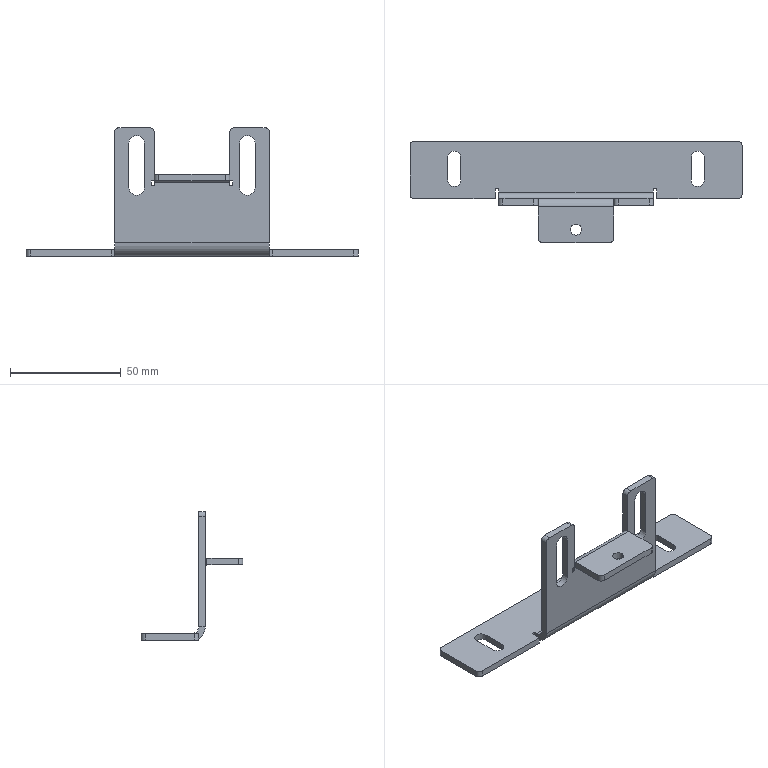Part | NX | features BREP 1 | 1 solid | 72 faces | box 150 x 46 x 58 mm | volume 21223 mm3 | plane 46 | cylinder 26 | commonest cylinder face diameters 4 x10 7 x6 6 x5 5 x2 1.473 x1 7.473 x1